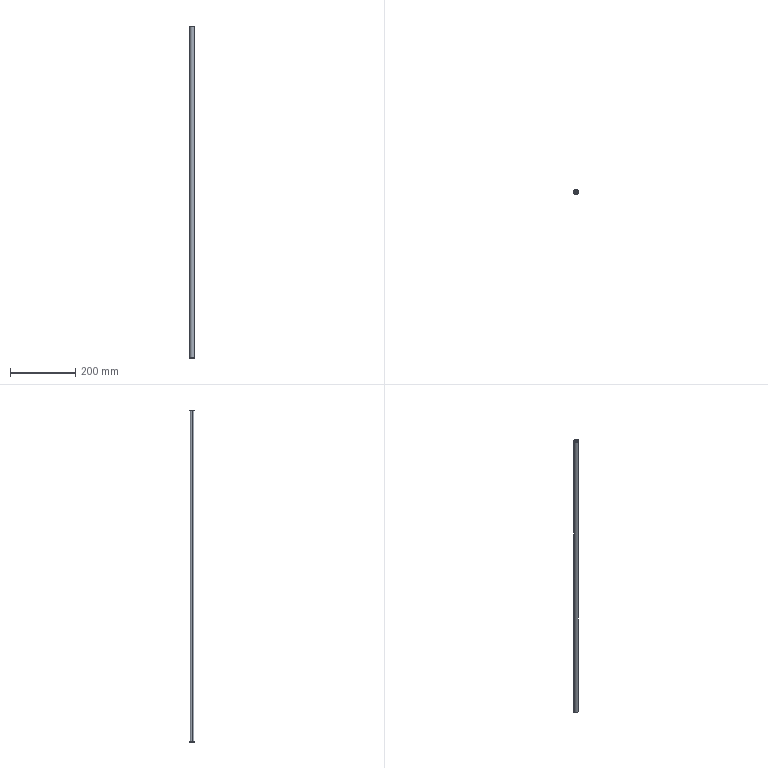Part | SolidWorks | features BaseBody 1 | 1 solid | 16 faces | box 15 x 15 x 1020 mm | volume 178720 mm3 | cone 8 | cylinder 6 | plane 2 | commonest cylinder face diameters 6.8 x4 15 x2
STEP:
#1=CARTESIAN_POINT('',(3.4,0.,-490.25));
#2=VERTEX_POINT('',#1);
#3=CARTESIAN_POINT('',(-3.4,0.,-490.25));
#4=VERTEX_POINT('',#3);
#5=CARTESIAN_POINT('',(0.,0.,-490.25));
#6=DIRECTION('',(0.,0.,-1.));
#7=DIRECTION('',(-1.,0.,0.));
#8=AXIS2_PLACEMENT_3D('',#5,#6,#7);
#9=CIRCLE('',#8,3.4);
#10=EDGE_CURVE('',#2,#4,#9,.T.);
#11=ORIENTED_EDGE('',*,*,#10,.F.);
#12=CARTESIAN_POINT('',(3.4,0.,-510.));
#13=VERTEX_POINT('',#12);
#14=CARTESIAN_POINT('',(3.4,0.,-510.));
#15=DIRECTION('',(0.,0.,-1.));
#16=VECTOR('',#15,1000.);
#17=LINE('',#14,#16);
#18=EDGE_CURVE('',#2,#13,#17,.T.);
#19=ORIENTED_EDGE('',*,*,#18,.T.);
#20=CARTESIAN_POINT('',(-3.4,0.,-510.));
#21=VERTEX_POINT('',#20);
#22=CARTESIAN_POINT('',(0.,0.,-510.));
#23=DIRECTION('',(0.,0.,-1.));
#24=DIRECTION('',(-1.,0.,0.));
#25=AXIS2_PLACEMENT_3D('',#22,#23,#24);
#26=CIRCLE('',#25,3.4);
#27=EDGE_CURVE('',#13,#21,#26,.T.);
#28=ORIENTED_EDGE('',*,*,#27,.T.);
#29=CARTESIAN_POINT('',(-3.4,0.,-510.));
#30=DIRECTION('',(0.,0.,-1.));
#31=VECTOR('',#30,1000.);
#32=LINE('',#29,#31);
#33=EDGE_CURVE('',#4,#21,#32,.T.);
#34=ORIENTED_EDGE('',*,*,#33,.F.);
#35=EDGE_LOOP('',(#11,#19,#28,#34));
#36=FACE_OUTER_BOUND('',#35,.T.);
#37=CARTESIAN_POINT('',(0.,0.,-510.));
#38=DIRECTION('',(0.,0.,-1.));
#39=DIRECTION('',(-1.,0.,0.));
#40=AXIS2_PLACEMENT_3D('',#37,#38,#39);
#41=CYLINDRICAL_SURFACE('',#40,3.4);
#42=ADVANCED_FACE('',(#36),#41,.F.);
#43=CARTESIAN_POINT('',(0.,0.,-488.207));
#44=VERTEX_POINT('',#43);
#45=CARTESIAN_POINT('',(-3.4,0.,-490.25));
#46=DIRECTION('',(-0.8572,0.,-0.515));
#47=VECTOR('',#46,1000.);
#48=LINE('',#45,#47);
#49=EDGE_CURVE('',#44,#4,#48,.T.);
#50=ORIENTED_EDGE('',*,*,#49,.F.);
#51=CARTESIAN_POINT('',(3.4,0.,-490.25));
#52=DIRECTION('',(0.8572,0.,-0.515));
#53=VECTOR('',#52,1000.);
#54=LINE('',#51,#53);
#55=EDGE_CURVE('',#44,#2,#54,.T.);
#56=ORIENTED_EDGE('',*,*,#55,.T.);
#57=ORIENTED_EDGE('',*,*,#10,.T.);
#58=EDGE_LOOP('',(#50,#56,#57));
#59=FACE_OUTER_BOUND('',#58,.T.);
#60=CARTESIAN_POINT('',(0.,0.,-490.25));
#61=DIRECTION('',(0.,0.,-1.));
#62=DIRECTION('',(-1.,0.,0.));
#63=AXIS2_PLACEMENT_3D('',#60,#61,#62);
#64=CONICAL_SURFACE('',#63,3.4,1.03);
#65=ADVANCED_FACE('',(#59),#64,.F.);
#66=CARTESIAN_POINT('',(-3.4,0.,490.25));
#67=VERTEX_POINT('',#66);
#68=CARTESIAN_POINT('',(3.4,0.,490.25));
#69=VERTEX_POINT('',#68);
#70=CARTESIAN_POINT('',(0.,0.,490.25));
#71=DIRECTION('',(0.,0.,1.));
#72=DIRECTION('',(1.,0.,0.));
#73=AXIS2_PLACEMENT_3D('',#70,#71,#72);
#74=CIRCLE('',#73,3.4);
#75=EDGE_CURVE('',#67,#69,#74,.T.);
#76=ORIENTED_EDGE('',*,*,#75,.F.);
#77=CARTESIAN_POINT('',(-3.4,0.,510.));
#78=VERTEX_POINT('',#77);
#79=CARTESIAN_POINT('',(-3.4,0.,510.));
#80=DIRECTION('',(0.,0.,1.));
#81=VECTOR('',#80,1000.);
#82=LINE('',#79,#81);
#83=EDGE_CURVE('',#67,#78,#82,.T.);
#84=ORIENTED_EDGE('',*,*,#83,.T.);
#85=CARTESIAN_POINT('',(3.4,0.,510.));
#86=VERTEX_POINT('',#85);
#87=CARTESIAN_POINT('',(0.,0.,510.));
#88=DIRECTION('',(0.,0.,1.));
#89=DIRECTION('',(1.,0.,0.));
#90=AXIS2_PLACEMENT_3D('',#87,#88,#89);
#91=CIRCLE('',#90,3.4);
#92=EDGE_CURVE('',#78,#86,#91,.T.);
#93=ORIENTED_EDGE('',*,*,#92,.T.);
#94=CARTESIAN_POINT('',(3.4,0.,510.));
#95=DIRECTION('',(0.,0.,1.));
#96=VECTOR('',#95,1000.);
#97=LINE('',#94,#96);
#98=EDGE_CURVE('',#69,#86,#97,.T.);
#99=ORIENTED_EDGE('',*,*,#98,.F.);
#100=EDGE_LOOP('',(#76,#84,#93,#99));
#101=FACE_OUTER_BOUND('',#100,.T.);
#102=CARTESIAN_POINT('',(0.,0.,510.));
#103=DIRECTION('',(0.,0.,1.));
#104=DIRECTION('',(1.,0.,0.));
#105=AXIS2_PLACEMENT_3D('',#102,#103,#104);
#106=CYLINDRICAL_SURFACE('',#105,3.4);
#107=ADVANCED_FACE('',(#101),#106,.F.);
#108=CARTESIAN_POINT('',(0.,0.,488.207));
#109=VERTEX_POINT('',#108);
#110=CARTESIAN_POINT('',(3.4,0.,490.25));
#111=DIRECTION('',(0.8572,0.,0.515));
#112=VECTOR('',#111,1000.);
#113=LINE('',#110,#112);
#114=EDGE_CURVE('',#109,#69,#113,.T.);
#115=ORIENTED_EDGE('',*,*,#114,.F.);
#116=CARTESIAN_POINT('',(-3.4,0.,490.25));
#117=DIRECTION('',(-0.8572,0.,0.515));
#118=VECTOR('',#117,1000.);
#119=LINE('',#116,#118);
#120=EDGE_CURVE('',#109,#67,#119,.T.);
#121=ORIENTED_EDGE('',*,*,#120,.T.);
#122=ORIENTED_EDGE('',*,*,#75,.T.);
#123=EDGE_LOOP('',(#115,#121,#122));
#124=FACE_OUTER_BOUND('',#123,.T.);
#125=CARTESIAN_POINT('',(0.,0.,490.25));
#126=DIRECTION('',(0.,0.,1.));
#127=DIRECTION('',(1.,0.,0.));
#128=AXIS2_PLACEMENT_3D('',#125,#126,#127);
#129=CONICAL_SURFACE('',#128,3.4,1.03);
#130=ADVANCED_FACE('',(#124),#129,.F.);
#131=CARTESIAN_POINT('',(6.5,0.,510.));
#132=VERTEX_POINT('',#131);
#133=CARTESIAN_POINT('',(-6.5,0.,510.));
#134=VERTEX_POINT('',#133);
#135=CARTESIAN_POINT('',(0.,0.,510.));
#136=DIRECTION('',(0.,0.,1.));
#137=DIRECTION('',(1.,0.,0.));
#138=AXIS2_PLACEMENT_3D('',#135,#136,#137);
#139=CIRCLE('',#138,6.5);
#140=EDGE_CURVE('',#132,#134,#139,.T.);
#141=ORIENTED_EDGE('',*,*,#140,.F.);
#142=CARTESIAN_POINT('',(7.5,0.,509.));
#143=VERTEX_POINT('',#142);
#144=CARTESIAN_POINT('',(6.5,0.,510.));
#145=DIRECTION('',(0.7071,0.,-0.7071));
#146=VECTOR('',#145,1000.);
#147=LINE('',#144,#146);
#148=EDGE_CURVE('',#132,#143,#147,.T.);
#149=ORIENTED_EDGE('',*,*,#148,.T.);
#150=CARTESIAN_POINT('',(-7.5,0.,509.));
#151=VERTEX_POINT('',#150);
#152=CARTESIAN_POINT('',(0.,0.,509.));
#153=DIRECTION('',(0.,0.,-1.));
#154=DIRECTION('',(1.,0.,0.));
#155=AXIS2_PLACEMENT_3D('',#152,#153,#154);
#156=CIRCLE('',#155,7.5);
#157=EDGE_CURVE('',#151,#143,#156,.T.);
#158=ORIENTED_EDGE('',*,*,#157,.F.);
#159=CARTESIAN_POINT('',(-6.5,0.,510.));
#160=DIRECTION('',(-0.7071,0.,-0.7071));
#161=VECTOR('',#160,1000.);
#162=LINE('',#159,#161);
#163=EDGE_CURVE('',#134,#151,#162,.T.);
#164=ORIENTED_EDGE('',*,*,#163,.F.);
#165=EDGE_LOOP('',(#141,#149,#158,#164));
#166=FACE_OUTER_BOUND('',#165,.T.);
#167=CARTESIAN_POINT('',(0.,0.,510.));
#168=DIRECTION('',(0.,0.,-1.));
#169=DIRECTION('',(-1.,0.,0.));
#170=AXIS2_PLACEMENT_3D('',#167,#168,#169);
#171=CONICAL_SURFACE('',#170,6.5,0.7854);
#172=ADVANCED_FACE('',(#166),#171,.T.);
#173=CARTESIAN_POINT('',(-6.5,0.,-510.));
#174=VERTEX_POINT('',#173);
#175=CARTESIAN_POINT('',(6.5,0.,-510.));
#176=VERTEX_POINT('',#175);
#177=CARTESIAN_POINT('',(0.,0.,-510.));
#178=DIRECTION('',(0.,0.,-1.));
#179=DIRECTION('',(1.,0.,0.));
#180=AXIS2_PLACEMENT_3D('',#177,#178,#179);
#181=CIRCLE('',#180,6.5);
#182=EDGE_CURVE('',#174,#176,#181,.T.);
#183=ORIENTED_EDGE('',*,*,#182,.F.);
#184=CARTESIAN_POINT('',(-7.5,0.,-509.));
#185=VERTEX_POINT('',#184);
#186=CARTESIAN_POINT('',(-7.5,0.,-509.));
#187=DIRECTION('',(-0.7071,0.,0.7071));
#188=VECTOR('',#187,1000.);
#189=LINE('',#186,#188);
#190=EDGE_CURVE('',#174,#185,#189,.T.);
#191=ORIENTED_EDGE('',*,*,#190,.T.);
#192=CARTESIAN_POINT('',(7.5,0.,-509.));
#193=VERTEX_POINT('',#192);
#194=CARTESIAN_POINT('',(0.,0.,-509.));
#195=DIRECTION('',(0.,0.,1.));
#196=DIRECTION('',(1.,0.,0.));
#197=AXIS2_PLACEMENT_3D('',#194,#195,#196);
#198=CIRCLE('',#197,7.5);
#199=EDGE_CURVE('',#193,#185,#198,.T.);
#200=ORIENTED_EDGE('',*,*,#199,.F.);
#201=CARTESIAN_POINT('',(7.5,0.,-509.));
#202=DIRECTION('',(0.7071,0.,0.7071));
#203=VECTOR('',#202,1000.);
#204=LINE('',#201,#203);
#205=EDGE_CURVE('',#176,#193,#204,.T.);
#206=ORIENTED_EDGE('',*,*,#205,.F.);
#207=EDGE_LOOP('',(#183,#191,#200,#206));
#208=FACE_OUTER_BOUND('',#207,.T.);
#209=CARTESIAN_POINT('',(0.,0.,-509.));
#210=DIRECTION('',(0.,0.,1.));
#211=DIRECTION('',(1.,0.,0.));
#212=AXIS2_PLACEMENT_3D('',#209,#210,#211);
#213=CONICAL_SURFACE('',#212,7.5,0.7854);
#214=ADVANCED_FACE('',(#208),#213,.T.);
#215=ORIENTED_EDGE('',*,*,#157,.T.);
#216=CARTESIAN_POINT('',(7.5,0.,510.));
#217=DIRECTION('',(0.,0.,-1.));
#218=VECTOR('',#217,1000.);
#219=LINE('',#216,#218);
#220=EDGE_CURVE('',#143,#193,#219,.T.);
#221=ORIENTED_EDGE('',*,*,#220,.T.);
#222=ORIENTED_EDGE('',*,*,#199,.T.);
#223=CARTESIAN_POINT('',(-7.5,0.,510.));
#224=DIRECTION('',(0.,0.,-1.));
#225=VECTOR('',#224,1000.);
#226=LINE('',#223,#225);
#227=EDGE_CURVE('',#151,#185,#226,.T.);
#228=ORIENTED_EDGE('',*,*,#227,.F.);
#229=EDGE_LOOP('',(#215,#221,#222,#228));
#230=FACE_OUTER_BOUND('',#229,.T.);
#231=CARTESIAN_POINT('',(0.,0.,510.));
#232=DIRECTION('',(0.,0.,-1.));
#233=DIRECTION('',(-1.,0.,0.));
#234=AXIS2_PLACEMENT_3D('',#231,#232,#233);
#235=CYLINDRICAL_SURFACE('',#234,7.5);
#236=ADVANCED_FACE('',(#230),#235,.T.);
#237=ORIENTED_EDGE('',*,*,#220,.F.);
#238=CARTESIAN_POINT('',(0.,0.,509.));
#239=DIRECTION('',(0.,0.,-1.));
#240=DIRECTION('',(1.,0.,0.));
#241=AXIS2_PLACEMENT_3D('',#238,#239,#240);
#242=CIRCLE('',#241,7.5);
#243=EDGE_CURVE('',#143,#151,#242,.T.);
#244=ORIENTED_EDGE('',*,*,#243,.T.);
#245=ORIENTED_EDGE('',*,*,#227,.T.);
#246=CARTESIAN_POINT('',(0.,0.,-509.));
#247=DIRECTION('',(0.,0.,1.));
#248=DIRECTION('',(1.,0.,0.));
#249=AXIS2_PLACEMENT_3D('',#246,#247,#248);
#250=CIRCLE('',#249,7.5);
#251=EDGE_CURVE('',#185,#193,#250,.T.);
#252=ORIENTED_EDGE('',*,*,#251,.T.);
#253=EDGE_LOOP('',(#237,#244,#245,#252));
#254=FACE_OUTER_BOUND('',#253,.T.);
#255=CARTESIAN_POINT('',(0.,0.,510.));
#256=DIRECTION('',(0.,0.,-1.));
#257=DIRECTION('',(-1.,0.,0.));
#258=AXIS2_PLACEMENT_3D('',#255,#256,#257);
#259=CYLINDRICAL_SURFACE('',#258,7.5);
#260=ADVANCED_FACE('',(#254),#259,.T.);
#261=CARTESIAN_POINT('',(0.,0.,510.));
#262=DIRECTION('',(0.,0.,1.));
#263=DIRECTION('',(1.,0.,0.));
#264=AXIS2_PLACEMENT_3D('',#261,#262,#263);
#265=CIRCLE('',#264,3.4);
#266=EDGE_CURVE('',#86,#78,#265,.T.);
#267=ORIENTED_EDGE('',*,*,#266,.F.);
#268=ORIENTED_EDGE('',*,*,#92,.F.);
#269=EDGE_LOOP('',(#267,#268));
#270=FACE_BOUND('',#269,.T.);
#271=CARTESIAN_POINT('',(0.,0.,510.));
#272=DIRECTION('',(0.,0.,1.));
#273=DIRECTION('',(1.,0.,0.));
#274=AXIS2_PLACEMENT_3D('',#271,#272,#273);
#275=CIRCLE('',#274,6.5);
#276=EDGE_CURVE('',#134,#132,#275,.T.);
#277=ORIENTED_EDGE('',*,*,#276,.T.);
#278=ORIENTED_EDGE('',*,*,#140,.T.);
#279=EDGE_LOOP('',(#277,#278));
#280=FACE_OUTER_BOUND('',#279,.T.);
#281=CARTESIAN_POINT('',(0.,0.,510.));
#282=DIRECTION('',(0.,0.,1.));
#283=DIRECTION('',(1.,0.,0.));
#284=AXIS2_PLACEMENT_3D('',#281,#282,#283);
#285=PLANE('',#284);
#286=ADVANCED_FACE('',(#270,#280),#285,.T.);
#287=CARTESIAN_POINT('',(0.,0.,-510.));
#288=DIRECTION('',(0.,0.,-1.));
#289=DIRECTION('',(-1.,0.,0.));
#290=AXIS2_PLACEMENT_3D('',#287,#288,#289);
#291=CIRCLE('',#290,3.4);
#292=EDGE_CURVE('',#21,#13,#291,.T.);
#293=ORIENTED_EDGE('',*,*,#292,.F.);
#294=ORIENTED_EDGE('',*,*,#27,.F.);
#295=EDGE_LOOP('',(#293,#294));
#296=FACE_BOUND('',#295,.T.);
#297=CARTESIAN_POINT('',(0.,0.,-510.));
#298=DIRECTION('',(0.,0.,-1.));
#299=DIRECTION('',(1.,0.,0.));
#300=AXIS2_PLACEMENT_3D('',#297,#298,#299);
#301=CIRCLE('',#300,6.5);
#302=EDGE_CURVE('',#176,#174,#301,.T.);
#303=ORIENTED_EDGE('',*,*,#302,.T.);
#304=ORIENTED_EDGE('',*,*,#182,.T.);
#305=EDGE_LOOP('',(#303,#304));
#306=FACE_OUTER_BOUND('',#305,.T.);
#307=CARTESIAN_POINT('',(0.,0.,-510.));
#308=DIRECTION('',(0.,0.,1.));
#309=DIRECTION('',(1.,0.,0.));
#310=AXIS2_PLACEMENT_3D('',#307,#308,#309);
#311=PLANE('',#310);
#312=ADVANCED_FACE('',(#296,#306),#311,.F.);
#313=ORIENTED_EDGE('',*,*,#190,.F.);
#314=ORIENTED_EDGE('',*,*,#302,.F.);
#315=ORIENTED_EDGE('',*,*,#205,.T.);
#316=ORIENTED_EDGE('',*,*,#251,.F.);
#317=EDGE_LOOP('',(#313,#314,#315,#316));
#318=FACE_OUTER_BOUND('',#317,.T.);
#319=CARTESIAN_POINT('',(0.,0.,-509.));
#320=DIRECTION('',(0.,0.,1.));
#321=DIRECTION('',(1.,0.,0.));
#322=AXIS2_PLACEMENT_3D('',#319,#320,#321);
#323=CONICAL_SURFACE('',#322,7.5,0.7854);
#324=ADVANCED_FACE('',(#318),#323,.T.);
#325=ORIENTED_EDGE('',*,*,#148,.F.);
#326=ORIENTED_EDGE('',*,*,#276,.F.);
#327=ORIENTED_EDGE('',*,*,#163,.T.);
#328=ORIENTED_EDGE('',*,*,#243,.F.);
#329=EDGE_LOOP('',(#325,#326,#327,#328));
#330=FACE_OUTER_BOUND('',#329,.T.);
#331=CARTESIAN_POINT('',(0.,0.,510.));
#332=DIRECTION('',(0.,0.,-1.));
#333=DIRECTION('',(-1.,0.,0.));
#334=AXIS2_PLACEMENT_3D('',#331,#332,#333);
#335=CONICAL_SURFACE('',#334,6.5,0.7854);
#336=ADVANCED_FACE('',(#330),#335,.T.);
#337=ORIENTED_EDGE('',*,*,#120,.F.);
#338=ORIENTED_EDGE('',*,*,#114,.T.);
#339=CARTESIAN_POINT('',(0.,0.,490.25));
#340=DIRECTION('',(0.,0.,1.));
#341=DIRECTION('',(1.,0.,0.));
#342=AXIS2_PLACEMENT_3D('',#339,#340,#341);
#343=CIRCLE('',#342,3.4);
#344=EDGE_CURVE('',#69,#67,#343,.T.);
#345=ORIENTED_EDGE('',*,*,#344,.T.);
#346=EDGE_LOOP('',(#337,#338,#345));
#347=FACE_OUTER_BOUND('',#346,.T.);
#348=CARTESIAN_POINT('',(0.,0.,490.25));
#349=DIRECTION('',(0.,0.,1.));
#350=DIRECTION('',(1.,0.,0.));
#351=AXIS2_PLACEMENT_3D('',#348,#349,#350);
#352=CONICAL_SURFACE('',#351,3.4,1.03);
#353=ADVANCED_FACE('',(#347),#352,.F.);
#354=ORIENTED_EDGE('',*,*,#83,.F.);
#355=ORIENTED_EDGE('',*,*,#344,.F.);
#356=ORIENTED_EDGE('',*,*,#98,.T.);
#357=ORIENTED_EDGE('',*,*,#266,.T.);
#358=EDGE_LOOP('',(#354,#355,#356,#357));
#359=FACE_OUTER_BOUND('',#358,.T.);
#360=CARTESIAN_POINT('',(0.,0.,510.));
#361=DIRECTION('',(0.,0.,1.));
#362=DIRECTION('',(1.,0.,0.));
#363=AXIS2_PLACEMENT_3D('',#360,#361,#362);
#364=CYLINDRICAL_SURFACE('',#363,3.4);
#365=ADVANCED_FACE('',(#359),#364,.F.);
#366=ORIENTED_EDGE('',*,*,#55,.F.);
#367=ORIENTED_EDGE('',*,*,#49,.T.);
#368=CARTESIAN_POINT('',(0.,0.,-490.25));
#369=DIRECTION('',(0.,0.,-1.));
#370=DIRECTION('',(-1.,0.,0.));
#371=AXIS2_PLACEMENT_3D('',#368,#369,#370);
#372=CIRCLE('',#371,3.4);
#373=EDGE_CURVE('',#4,#2,#372,.T.);
#374=ORIENTED_EDGE('',*,*,#373,.T.);
#375=EDGE_LOOP('',(#366,#367,#374));
#376=FACE_OUTER_BOUND('',#375,.T.);
#377=CARTESIAN_POINT('',(0.,0.,-490.25));
#378=DIRECTION('',(0.,0.,-1.));
#379=DIRECTION('',(-1.,0.,0.));
#380=AXIS2_PLACEMENT_3D('',#377,#378,#379);
#381=CONICAL_SURFACE('',#380,3.4,1.03);
#382=ADVANCED_FACE('',(#376),#381,.F.);
#383=ORIENTED_EDGE('',*,*,#18,.F.);
#384=ORIENTED_EDGE('',*,*,#373,.F.);
#385=ORIENTED_EDGE('',*,*,#33,.T.);
#386=ORIENTED_EDGE('',*,*,#292,.T.);
#387=EDGE_LOOP('',(#383,#384,#385,#386));
#388=FACE_OUTER_BOUND('',#387,.T.);
#389=CARTESIAN_POINT('',(0.,0.,-510.));
#390=DIRECTION('',(0.,0.,-1.));
#391=DIRECTION('',(-1.,0.,0.));
#392=AXIS2_PLACEMENT_3D('',#389,#390,#391);
#393=CYLINDRICAL_SURFACE('',#392,3.4);
#394=ADVANCED_FACE('',(#388),#393,.F.);
#395=CLOSED_SHELL('',(#42,#65,#107,#130,#172,#214,#236,#260,#286,#312,#324,#336,#353,#365,#382,#394));
#396=MANIFOLD_SOLID_BREP('',#395);
#397=CARTESIAN_POINT('',(0.,0.,0.));
#398=DIRECTION('',(0.,0.,1.));
#399=DIRECTION('',(1.,0.,0.));
#400=AXIS2_PLACEMENT_3D('',#397,#398,#399);
#401=(LENGTH_UNIT()NAMED_UNIT(*)SI_UNIT(.MILLI.,.METRE.));
#402=UNCERTAINTY_MEASURE_WITH_UNIT(LENGTH_MEASURE(0.00001),#401,'','');
#403=(NAMED_UNIT(*)PLANE_ANGLE_UNIT()SI_UNIT($,.RADIAN.));
#404=(NAMED_UNIT(*)SI_UNIT($,.STERADIAN.)SOLID_ANGLE_UNIT());
#405=(GEOMETRIC_REPRESENTATION_CONTEXT(3)GLOBAL_UNCERTAINTY_ASSIGNED_CONTEXT((#402))GLOBAL_UNIT_ASSIGNED_CONTEXT((#401,#403,#404))REPRESENTATION_CONTEXT('',''));
#406=ADVANCED_BREP_SHAPE_REPRESENTATION('',(#396,#400),#405);